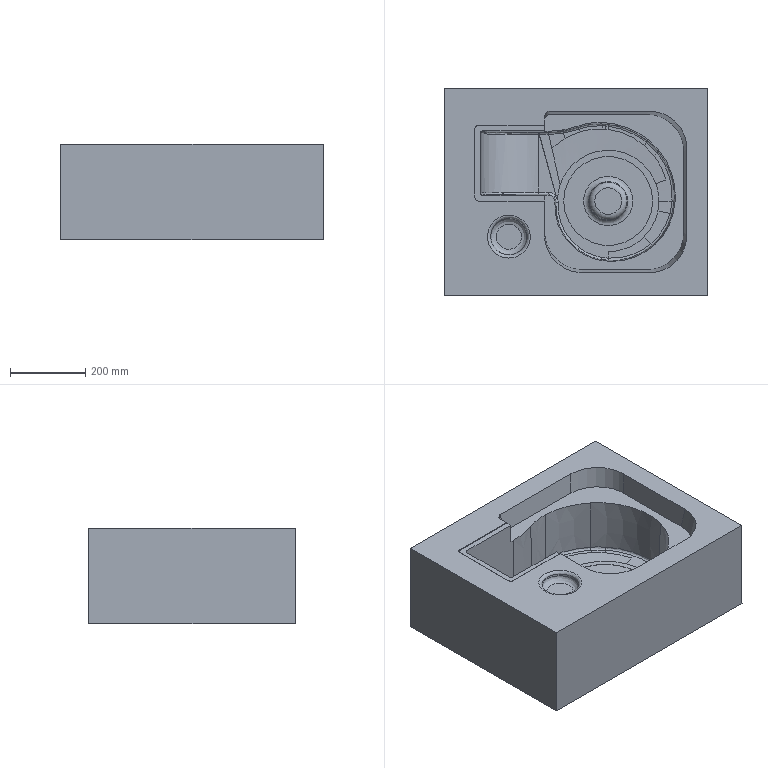NC program | NX | posted with a generic post | part box 700 x 550 x 255 mm
Lines 17668 to 18915 of 43405:
(CAVITY_MILL_COPY_1 , TOOL : D26R0.8)
N35328 M6
N35330 G54
N35332 G17 G0 G90 X-44.068 Y188.604 S1000 M3
N35334 G43 Z30. H0
N35336 Z0.302
N35338 G94 G1 Z-0.698 F1800.
N35340 Y201.604
N35342 X-57.068
N35344 X-68.784
N35346 G3 X-70.358 Y200.391 R1.628
N35348 X-70.433 Y199.808 R2.293
N35350 G1 Y188.61
N35352 Y154.444
N35354 Z0.302
N35356 G0 Z3.
N35358 X-39.123 Y188.506
N35360 Z-0.396
N35362 G1 Z-1.396
N35364 Y201.506
N35366 X-52.123
N35368 X-68.766
N35370 G3 X-70.382 Y200.106 R1.633
N35372 X-70.423 Y199.452 R4.078
N35374 G1 Y184.498
N35376 Y153.351
N35378 Z-0.396
N35380 G0 Z2.302
N35382 X-39.117 Y188.408
N35384 Z-1.094
N35386 G1 Z-2.094
N35388 Y201.408
N35390 X-52.117
N35392 X-68.787
N35394 G3 X-70.356 Y200.026 R1.582
N35396 G1 X-70.408 Y199.618
N35398 X-70.417 Y199.467
N35400 Y184.4
N35402 Y140.492
N35404 Z-1.094
N35406 G0 Z1.604
N35408 X-39.111 Y188.31
N35410 Z-1.792
N35412 G1 Z-2.792
N35414 Y201.31
N35416 X-52.111
N35418 X-68.759
N35420 G3 X-70.37 Y199.838 R1.617
N35422 G1 X-70.411 Y199.386
N35424 Y184.302
N35426 Y139.998
N35428 Z-1.792
N35430 G0 Z0.906
N35432 X-39.105 Y188.212
N35434 Z-2.491
N35436 G1 Z-3.491
N35438 Y201.212
N35440 X-52.105
N35442 X-68.755
N35444 G3 X-70.357 Y199.752 R1.609
N35446 G1 X-70.405 Y199.243
N35448 Y184.204
N35450 Y139.977
N35452 Z-2.491
N35454 G0 Z0.208
N35456 X-39.099 Y188.114
N35458 Z-3.189
N35460 G1 Z-4.189
N35462 Y201.114
N35464 X-52.099
N35466 X-68.745
N35468 G3 X-70.353 Y199.654 R1.615
N35470 G1 X-70.399 Y199.181
N35472 Y184.106
N35474 Y139.965
N35476 Z-3.189
N35478 G0 Z-0.491
N35480 X-39.093 Y188.016
N35482 Z-3.887
N35484 G1 Z-4.887
N35486 Y201.016
N35488 X-52.093
N35490 X-68.749
N35492 G3 X-70.334 Y199.669 R1.606
N35494 X-70.392 Y198.978 R4.518
N35496 G1 Y184.008
N35498 Y139.953
N35500 Z-3.887
N35502 G0 Z-1.189
N35504 X-39.087 Y187.918
N35506 Z-4.585
N35508 G1 Z-5.585
N35510 Y200.918
N35512 X-52.087
N35514 X-68.711
N35516 G3 X-70.358 Y199.38 R1.652
N35518 G1 X-70.386 Y198.974
N35520 Y183.91
N35522 Y139.94
N35524 Z-4.585
N35526 G0 Z-1.887
N35528 X-39.08 Y187.82
N35530 Z-5.283
N35532 G1 Z-6.283
N35534 Y200.82
N35536 X-52.08
N35538 X-68.721
N35540 G3 X-70.33 Y199.468 R1.633
N35542 G1 X-70.349 Y199.357
N35544 X-70.38 Y198.756
N35546 Y183.811
N35548 Y139.928
N35550 Z-5.283
N35552 G0 Z-2.585
N35554 X-39.074 Y187.721
N35556 Z-5.981
N35558 G1 Z-6.981
N35560 Y200.721
N35562 X-52.074
N35564 X-68.709
N35566 G3 X-70.265 Y199.577 R1.63
N35568 G1 X-70.314 Y199.418
N35570 X-70.374 Y198.752
N35572 Y183.713
N35574 Y139.922
N35576 Z-5.981
N35578 G0 Z-3.283
N35580 X-39.068 Y187.623
N35582 Z-6.679
N35584 G1 Z-7.679
N35586 Y200.623
N35588 X-52.068
N35590 X-68.695
N35592 G3 X-70.305 Y199.312 R1.644
N35594 G1 X-70.332 Y199.181
N35596 X-70.368 Y198.583
N35598 Y183.615
N35600 Y139.911
N35602 Z-6.679
N35604 G0 Z-3.981
N35606 X-39.062 Y187.525
N35608 Z-7.377
N35610 G1 Z-8.377
N35612 Y200.525
N35614 X-52.062
N35616 X-68.709
N35618 G3 X-70.316 Y199.062 R1.615
N35620 G1 X-70.362 Y198.579
N35622 Y183.517
N35624 Y139.892
N35626 Z-7.377
N35628 G0 Z-4.679
N35630 X-39.056 Y187.427
N35632 Z-8.076
N35634 G1 Z-9.076
N35636 Y200.427
N35638 X-52.056
N35640 X-68.686
N35642 G3 X-70.289 Y199.1 R1.632
N35644 X-70.356 Y198.378 R3.795
N35646 G1 Y183.419
N35648 Y139.879
N35650 Z-8.076
N35652 G0 Z-5.377
N35654 X-39.05 Y187.329
N35656 Z-8.774
N35658 G1 Z-9.774
N35660 Y200.329
N35662 X-52.05
N35664 X-68.679
N35666 G3 X-70.264 Y199.083 R1.63
N35668 X-70.35 Y198.374 R3.058
N35670 G1 Y183.321
N35672 Y139.867
N35674 Z-8.774
N35676 G0 Z-6.076
N35678 X-39.044 Y187.231
N35680 Z-9.472
N35682 G1 Z-10.472
N35684 Y200.231
N35686 X-52.044
N35688 X-68.677
N35690 G3 X-70.221 Y199.106 R1.622
N35692 X-70.344 Y198.371 R2.564
N35694 G1 Y183.223
N35696 Y139.855
N35698 Z-9.472
N35700 G0 Z-6.774
N35702 X-39.038 Y187.133
N35704 Z-10.17
N35706 G1 Z-11.17
N35708 Y200.133
N35710 X-52.038
N35712 X-68.663
N35714 G3 X-70.268 Y198.777 R1.628
N35716 G1 X-70.338 Y198.367
N35718 Y183.125
N35720 Y139.843
N35722 Z-10.17
N35724 G0 Z-7.472
N35726 X-39.032 Y187.035
N35728 Z-10.868
N35730 G1 Z-11.868
N35732 Y200.035
N35734 X-52.032
N35736 X-68.655
N35738 G3 X-70.256 Y198.746 R1.638
N35740 X-70.332 Y197.924 R3.364
N35742 G1 Y183.027
N35744 Y139.831
N35746 Z-10.868
N35748 G0 Z-8.17
N35750 X-39.026 Y186.937
N35752 Z-11.566
N35754 G1 Z-12.566
N35756 Y199.937
N35758 X-52.026
N35760 X-68.651
N35762 G3 X-70.257 Y198.601 R1.633
N35764 X-70.325 Y197.924 R4.148
N35766 G1 Y182.928
N35768 Y139.818
N35770 Z-11.566
N35772 G0 Z-8.868
N35774 X-39.02 Y186.838
N35776 Z-12.264
N35778 G1 Z-13.264
N35780 Y199.838
N35782 X-52.02
N35784 X-68.643
N35786 G3 X-70.268 Y198.384 R1.635
N35788 G1 X-70.319 Y197.924
N35790 Y182.83
N35792 Y139.806
N35794 Z-12.264
N35796 G0 Z-9.566
N35798 X-39.013 Y186.74
N35800 Z-12.962
N35802 G1 Z-13.962
N35804 Y199.74
N35806 X-52.013
N35808 X-68.637
N35810 G3 X-70.257 Y198.284 R1.63
N35812 G1 X-70.296 Y197.924
N35814 X-70.313 Y197.889
N35816 Y182.732
N35818 Y139.794
N35820 Z-12.962
N35822 G0 Z-10.264
N35824 X-39.007 Y186.642
N35826 Z-13.66
N35828 G1 Z-14.66
N35830 Y199.642
N35832 X-52.007
N35834 X-68.631
N35836 G3 X-70.243 Y198.242 R1.628
N35838 G1 X-70.307 Y197.789
N35840 Y182.634
N35842 Y139.782
N35844 Z-13.66
N35846 G0 Z-10.962
N35848 X-39.001 Y186.544
N35850 Z-14.359
N35852 G1 Z-15.359
N35854 Y199.544
N35856 X-52.001
N35858 X-68.614
N35860 G3 X-70.236 Y198.139 R1.639
N35862 G1 X-70.301 Y197.69
N35864 Y182.536
N35866 Y139.77
N35868 Z-14.359
N35870 G0 Z-11.66
N35872 X-38.995 Y186.446
N35874 Z-15.057
N35876 G1 Z-16.057
N35878 Y199.446
N35880 X-51.995
N35882 X-68.653
N35884 G3 X-70.198 Y198.147 R1.568
N35886 G1 X-70.295 Y197.59
N35888 Y182.438
N35890 Y139.758
N35892 Z-15.057
N35894 G0 Z-12.359
N35896 X-38.989 Y186.348
N35898 Z-15.755
N35900 G1 Z-16.755
N35902 Y199.348
N35904 X-51.989
N35906 X-68.507
N35908 G3 X-70.054 Y198.463 R1.634
N35910 X-70.289 Y197.491 R2.485
N35912 G1 Y182.34
N35914 Y139.745
N35916 Z-15.755
N35918 G0 Z-13.057
N35920 X-38.983 Y186.25
N35922 Z-16.453
N35924 G1 Z-17.453
N35926 Y199.25
N35928 X-51.983
N35930 X-68.606
N35932 G3 X-70.077 Y198.296 R1.611
N35934 G1 X-70.086 Y198.276
N35936 G3 X-70.283 Y197.391 R1.86
N35938 G1 Y182.242
N35940 Y139.733
N35942 Z-16.453
N35944 G0 Z-13.755
N35946 X-38.977 Y186.152
N35948 Z-17.151
N35950 G1 Z-18.151
N35952 Y199.152
N35954 X-51.977
N35956 X-68.494
N35958 G3 X-70.044 Y198.26 R1.634
N35960 X-70.277 Y197.292 R1.961
N35962 G1 Y182.144
N35964 Y139.721
N35966 Z-17.151
N35968 G0 Z-14.453
N35970 X-38.971 Y186.054
N35972 Z-17.849
N35974 G1 Z-18.849
N35976 Y199.054
N35978 X-51.971
N35980 X-68.488
N35982 G3 X-70.132 Y197.924 R1.623
N35984 X-70.271 Y197.192 R1.509
N35986 G1 Y182.045
N35988 Y139.709
N35990 Z-17.849
N35992 G0 Z-15.151
N35994 X-38.965 Y185.955
N35996 Z-18.547
N35998 G1 Z-19.547
N36000 Y198.955
N36002 X-51.965
N36004 X-68.482
N36006 G3 X-69.579 Y198.623 R1.753
N36008 X-70.264 Y197.093 R1.952
N36010 G1 Y181.947
N36012 Y139.697
N36014 Z-18.547
N36016 G0 Z-15.849
N36018 X-38.959 Y185.857
N36020 Z-19.245
N36022 G1 Z-20.245
N36024 Y198.857
N36026 X-51.959
N36028 X-68.598
N36030 G3 X-69.901 Y198.173 R1.583
N36032 X-70.258 Y196.994 R2.026
N36034 G1 Y181.849
N36036 Y139.691
N36038 Z-19.245
N36040 G0 Z-16.547
N36042 X-38.953 Y185.759
N36044 Z-19.943
N36046 G1 Z-20.943
N36048 Y198.759
N36050 X-51.953
N36052 X-68.545
N36054 G3 X-70.206 Y197.285 R1.673
N36056 G1 X-70.252 Y196.894
N36058 Y181.751
N36060 Y139.68
N36062 Z-19.943
N36064 G0 Z-17.245
N36066 X-38.946 Y185.661
N36068 Z-20.642
N36070 G1 Z-21.642
N36072 Y198.661
N36074 X-51.946
N36076 X-68.554
N36078 G3 X-70.198 Y197.162 R1.65
N36080 G1 X-70.231 Y196.795
N36082 X-70.246 Y196.667
N36084 Y181.653
N36086 Y139.66
N36088 Z-20.642
N36090 G0 Z-17.943
N36092 X-38.94 Y185.563
N36094 Z-21.34
N36096 G1 Z-22.34
N36098 Y198.563
N36100 X-51.94
N36102 X-68.547
N36104 G3 X-70.191 Y197.063 R1.651
N36106 G1 X-70.225 Y196.695
N36108 X-70.24 Y196.667
N36110 Y181.555
N36112 Y139.648
N36114 Z-21.34
N36116 G0 Z-18.642
N36118 X-38.934 Y185.465
N36120 Z-22.038
N36122 G1 Z-23.038
N36124 Y198.465
N36126 X-51.934
N36128 X-68.534
N36130 G3 X-70.186 Y196.967 R1.66
N36132 G1 X-70.215 Y196.667
N36134 X-70.234 Y196.575
N36136 Y181.457
N36138 Y139.636
N36140 Z-22.038
N36142 G0 Z-19.34
N36144 X-38.928 Y185.367
N36146 Z-22.736
N36148 G1 Z-23.736
N36150 Y198.367
N36152 X-51.928
N36154 X-68.555
N36156 G3 X-70.176 Y196.925 R1.632
N36158 G1 X-70.228 Y196.48
N36160 Y181.359
N36162 Y139.624
N36164 Z-22.736
N36166 G0 Z-20.038
N36168 X-38.922 Y185.269
N36170 Z-23.434
N36172 G1 Z-24.434
N36174 Y198.269
N36176 X-51.922
N36178 X-68.547
N36180 G3 X-70.169 Y196.828 R1.633
N36182 G1 X-70.222 Y196.384
N36184 Y181.261
N36186 Y139.611
N36188 Z-23.434
N36190 G0 Z-20.736
N36192 X-38.916 Y185.171
N36194 Z-24.132
N36196 G1 Z-25.132
N36198 Y198.171
N36200 X-51.916
N36202 X-68.433
N36204 G3 X-70.174 Y196.667 R1.668
N36206 G1 X-70.216 Y196.289
N36208 Y181.162
N36210 Y139.599
N36212 Z-24.132
N36214 G0 Z-21.434
N36216 X-38.91 Y185.072
N36218 Z-24.83
N36220 G1 Z-25.83
N36222 Y198.072
N36224 X-51.91
N36226 X-68.427
N36228 G3 X-70.161 Y196.639 R1.67
N36230 G1 X-70.21 Y196.193
N36232 Y181.064
N36234 Y139.587
N36236 Z-24.83
N36238 G0 Z-22.132
N36240 X-38.904 Y184.974
N36242 Z-25.528
N36244 G1 Z-26.528
N36246 Y197.974
N36248 X-51.904
N36250 X-68.522
N36252 G3 X-70.061 Y196.884 R1.631
N36254 X-70.204 Y196.098 R2.538
N36256 G1 Y180.966
N36258 Y139.575
N36260 Z-25.528
N36262 G0 Z-22.83
N36264 X-38.898 Y184.876
N36266 Z-26.227
N36268 G1 Z-27.227
N36270 Y197.876
N36272 X-51.898
N36274 X-68.51
N36276 G3 X-70.064 Y196.753 R1.637
N36278 X-70.197 Y196.003 R2.655
N36280 G1 Y180.868
N36282 Y139.563
N36284 Z-26.227
N36286 G0 Z-23.528
N36288 X-38.892 Y184.778
N36290 Z-26.925
N36292 G1 Z-27.925
N36294 Y197.778
N36296 X-51.892
N36298 X-68.508
N36300 G3 X-70.055 Y196.665 R1.632
N36302 X-70.191 Y195.907 R2.639
N36304 G1 Y180.77
N36306 Y139.55
N36308 Z-26.925
N36310 G0 Z-24.227
N36312 X-38.886 Y184.68
N36314 Z-27.623
N36316 G1 Z-28.623
N36318 Y197.68
N36320 X-51.886
N36322 X-68.5
N36324 G3 X-70.048 Y196.575 R1.637
N36326 X-70.185 Y195.812 R2.55
N36328 G1 Y180.672
N36330 Y139.538
N36332 Z-27.623
N36334 G0 Z-24.925
N36336 X-38.879 Y184.582
N36338 Z-28.321
N36340 G1 Z-29.321
N36342 Y197.582
N36344 X-51.879
N36346 X-68.397
N36348 G3 X-69.998 Y196.596 R1.654
N36350 X-70.179 Y195.716 R2.546
N36352 G1 Y180.574
N36354 Y139.526
N36356 Z-28.321
N36358 G0 Z-25.623
N36360 X-38.873 Y184.484
N36362 Z-29.019
N36364 G1 Z-30.019
N36366 Y197.484
N36368 X-51.873
N36370 X-68.482
N36372 G3 X-70.046 Y196.35 R1.647
N36374 X-70.173 Y195.621 R2.564
N36376 G1 Y180.476
N36378 Y139.514
N36380 Z-29.019
N36382 G0 Z-26.321
N36384 X-38.867 Y184.386
N36386 Z-29.717
N36388 G1 Z-30.717
N36390 Y197.386
N36392 X-51.867
N36394 X-68.475
N36396 G3 X-70.045 Y196.24 R1.649
N36398 X-70.167 Y195.411 R2.568
N36400 G1 Y180.377
N36402 Y139.502
N36404 Z-29.717
N36406 G0 Z-27.019
N36408 X-38.861 Y184.287
N36410 Z-30.415
N36412 G1 Z-31.415
N36414 Y197.287
N36416 X-51.861
N36418 X-68.379
N36420 G3 X-69.998 Y196.263 R1.661
N36422 X-70.161 Y195.411 R2.598
N36424 G1 Y180.279
N36426 Y139.489
N36428 Z-30.415
N36430 G0 Z-27.717
N36432 X-38.855 Y184.189
N36434 Z-31.113
N36436 G1 Z-32.113
N36438 Y197.189
N36440 X-51.855
N36442 X-68.372
N36444 G3 X-70.106 Y195.762 R1.676
N36446 G1 X-70.155 Y195.244
N36448 Y180.181
N36450 Y139.477
N36452 Z-31.113
N36454 G0 Z-28.415
N36456 X-38.849 Y184.091
N36458 Z-31.811
N36460 G1 Z-32.811
N36462 Y197.091
N36464 X-51.849
N36466 X-68.366
N36468 G3 X-70.1 Y195.664 R1.674
N36470 G1 X-70.149 Y195.158
N36472 Y180.083
N36474 Y139.465
N36476 Z-31.811
N36478 G0 Z-29.113
N36480 X-38.843 Y183.993
N36482 Z-32.51
N36484 G1 Z-33.51
N36486 Y196.993
N36488 X-51.843
N36490 X-68.36
N36492 G3 X-70.094 Y195.567 R1.674
N36494 G1 X-70.132 Y195.156
N36496 X-70.143 Y195.072
N36498 Y179.985
N36500 Y139.453
N36502 Z-32.51
N36504 G0 Z-29.811
N36506 X-38.837 Y183.895
N36508 Z-33.208
N36510 G1 Z-34.208
N36512 Y196.895
N36514 X-51.837
N36516 X-68.354
N36518 G3 X-70.088 Y195.469 R1.671
N36520 G1 X-70.137 Y195.002
N36522 Y179.887
N36524 Y139.441
N36526 Z-33.208
N36528 G0 Z-30.51
N36530 X-38.831 Y183.797
N36532 Z-33.906
N36534 G1 Z-34.906
N36536 Y196.797
N36538 X-51.831
N36540 X-68.348
N36542 G3 X-70.072 Y195.411 R1.663
N36544 G1 X-70.13 Y195.
N36546 Y179.789
N36548 Y139.429
N36550 Z-33.906
N36552 G0 Z-31.208
N36554 X-38.825 Y183.699
N36556 Z-34.604
N36558 G1 Z-35.604
N36560 Y196.699
N36562 X-51.825
N36564 X-68.46
N36566 G3 X-70.057 Y195.3 R1.61
N36568 G1 X-70.124 Y194.791
N36570 Y179.691
N36572 Y139.416
N36574 Z-34.604
N36576 G0 Z-31.906
N36578 X-38.819 Y183.601
N36580 Z-35.302
N36582 G1 Z-36.302
N36584 Y196.601
N36586 X-51.819
N36588 X-68.43
N36590 G3 X-70.042 Y195.208 R1.628
N36592 G1 X-70.118 Y194.685
N36594 Y179.593
N36596 Y139.404
N36598 Z-35.302
N36600 G0 Z-32.604
N36602 X-38.812 Y183.503
N36604 Z-36.
N36606 G1 Z-37.
N36608 Y196.503
N36610 X-51.812
N36612 X-68.33
N36614 G3 X-70.063 Y194.993 R1.646
N36616 G1 X-70.112 Y194.631
N36618 Y179.494
N36620 Y139.392
N36622 Z-36.
N36624 G0 Z-33.302
N36626 X-38.806 Y183.404
N36628 Z-36.698
N36630 G1 Z-37.698
N36632 Y196.404
N36634 X-51.806
N36636 X-68.324
N36638 G3 X-70.043 Y194.99 R1.64
N36640 G1 X-70.106 Y194.502
N36642 Y179.396
N36644 Y139.38
N36646 Z-36.698
N36648 G0 Z-34.
N36650 X-38.8 Y183.306
N36652 Z-37.396
N36654 G1 Z-38.396
N36656 Y196.306
N36658 X-51.8
N36660 X-68.417
N36662 G3 X-70.035 Y194.897 R1.633
N36664 G1 X-70.1 Y194.424
N36666 Y179.298
N36668 Y139.368
N36670 Z-37.396
N36672 G0 Z-34.698
N36674 X-38.794 Y183.208
N36676 Z-38.095
N36678 G1 Z-39.095
N36680 Y196.208
N36682 X-51.794
N36684 X-68.403
N36686 G3 X-70.027 Y194.804 R1.641
N36688 G1 X-70.094 Y194.346
N36690 Y179.2
N36692 Y139.355
N36694 Z-38.095
N36696 G0 Z-35.396
N36698 X-38.788 Y183.11
N36700 Z-38.793
N36702 G1 Z-39.793
N36704 Y196.11
N36706 X-51.788
N36708 X-68.404
N36710 G3 X-70.028 Y194.679 R1.637
N36712 G1 X-70.088 Y194.211
N36714 Y179.102
N36716 Y139.343
N36718 Z-38.793
N36720 G0 Z-36.095
N36722 X-38.782 Y183.012
N36724 Z-39.491
N36726 G1 Z-40.491
N36728 Y196.012
N36730 X-51.782
N36732 X-68.299
N36734 G3 X-70.037 Y194.492 R1.652
N36736 G1 X-70.082 Y194.121
N36738 Y179.004
N36740 Y139.331
N36742 Z-39.491
N36744 G0 Z-36.793
N36746 X-38.776 Y182.914
N36748 Z-40.189
N36750 G1 Z-41.189
N36752 Y195.914
N36754 X-51.776
N36756 X-68.394
N36758 G3 X-70.02 Y194.496 R1.641
N36760 G1 X-70.021 Y194.49
N36762 X-70.038 Y194.415
N36764 X-70.076 Y194.02
N36766 Y178.906
N36768 Y139.319
N36770 Z-40.189
N36772 G0 Z-37.491
N36774 X-38.77 Y182.816
N36776 Z-40.887
N36778 G1 Z-41.887
N36780 Y195.816
N36782 X-51.77
N36784 X-68.287
N36786 G3 X-70.033 Y194.261 R1.658
N36788 G1 X-70.07 Y193.952
N36790 Y178.808
N36792 Y139.307
N36794 Z-40.887
N36796 G0 Z-38.189
N36798 X-38.764 Y182.718
N36800 Z-41.585
N36802 G1 Z-42.585
N36804 Y195.718
N36806 X-51.764
N36808 X-68.281
N36810 G3 X-70.017 Y194.259 R1.649
N36812 G1 X-70.063 Y193.824
N36814 Y178.71
N36816 Y139.295
N36818 Z-41.585
N36820 G0 Z-38.887
N36822 X-38.758 Y182.62
N36824 Z-42.283
N36826 G1 Z-43.283
N36828 Y195.62
N36830 X-51.758
N36832 X-68.275
N36834 G3 X-70.014 Y194.154 R1.654
N36836 G1 X-70.057 Y193.762
N36838 Y178.611
N36840 Y139.282
N36842 Z-42.283
N36844 G0 Z-39.585
N36846 X-38.752 Y182.521
N36848 Z-42.981
N36850 G1 Z-43.981
N36852 Y195.521
N36854 X-51.752
N36856 X-68.386
N36858 G3 X-69.828 Y194.615 R1.601
N36860 X-70.051 Y193.639 R2.254
N36862 G1 Y178.513
N36864 Y139.27
N36866 Z-42.981
N36868 G0 Z-40.283
N36870 X-38.745 Y182.423
N36872 Z-43.679
N36874 G1 Z-44.679
N36876 Y195.423
N36878 X-51.745
N36880 X-68.263
N36882 G3 X-70.015 Y193.883 R1.664
N36884 G1 X-70.045 Y193.512
N36886 Y178.415
N36888 Y139.258
N36890 Z-43.679
N36892 G0 Z-40.981
N36894 X-38.739 Y182.325
N36896 Z-44.378
N36898 G1 Z-45.378
N36900 Y195.325
N36902 X-51.739
N36904 X-68.366
N36906 G3 X-69.931 Y194.158 R1.633
N36908 X-70.039 Y193.449 R2.598
N36910 G1 Y178.317
N36912 Y139.246
N36914 Z-44.378
N36916 G0 Z-41.679
N36918 X-38.733 Y182.227
N36920 Z-45.076
N36922 G1 Z-46.076
N36924 Y195.227
N36926 X-51.733
N36928 X-68.25
N36930 G3 X-69.998 Y193.789 R1.666
N36932 G1 X-70.033 Y193.387
N36934 Y178.219
N36936 Y139.234
N36938 Z-45.076
N36940 G0 Z-42.378
N36942 X-38.727 Y182.129
N36944 Z-45.774
N36946 G1 Z-46.774
N36948 Y195.129
N36950 X-51.727
N36952 X-68.345
N36954 G3 X-69.973 Y193.773 R1.656
N36956 G1 X-69.998 Y193.639
N36958 X-70.027 Y193.229
N36960 Y178.121
N36962 Y139.221
N36964 Z-45.774
N36966 G0 Z-43.076
N36968 X-38.721 Y182.031
N36970 Z-46.472
N36972 G1 Z-47.472
N36974 Y195.031
N36976 X-51.721
N36978 X-68.347
N36980 G3 X-69.968 Y193.615 R1.637
N36982 G1 X-70.021 Y193.229
N36984 Y178.023
N36986 Y139.209
N36988 Z-46.472
N36990 G0 Z-43.774
N36992 X-38.715 Y181.933
N36994 Z-47.17
N36996 G1 Z-48.17
N36998 Y194.933
N37000 X-51.715
N37002 X-68.342
N37004 G3 X-69.931 Y193.69 R1.637
N37006 X-70.015 Y193.025 R2.846
N37008 G1 Y177.925
N37010 Y139.197
N37012 Z-47.17
N37014 G0 Z-44.472
N37016 X-38.709 Y181.835
N37018 Z-47.868
N37020 G1 Z-48.868
N37022 Y194.835
N37024 X-51.709
N37026 X-68.332
N37028 G3 X-69.965 Y193.386 R1.644
N37030 G1 X-70.009 Y193.024
N37032 Y177.827
N37034 Y139.185
N37036 Z-47.868
N37038 G0 Z-45.17
N37040 X-38.703 Y181.737
N37042 Z-48.566
N37044 G1 Z-49.566
N37046 Y194.737
N37048 X-51.703
N37050 X-68.369
N37052 G3 X-69.906 Y193.46 R1.564
N37054 G1 X-69.998 Y192.973
N37056 X-70.003 Y192.897
N37058 Y177.728
N37060 Y139.173
N37062 Z-48.566
N37064 G0 Z3.
N37066 X-57.9 Y172.249
N37068 Z0.302
N37070 G1 Z-0.698
N37072 X-79.312 Y164.576
N37074 G2 X-83.957 Y163.792 R13.398
N37076 G1 X-256.512
N37078 Y-10.819
N37080 X-83.845
N37082 G2 X-79.452 Y-11.561 R13.419
N37084 G1 X-57.953 Y-19.024
N37086 Z0.302
N37088 G0 Z3.
N37090 X-57.281 Y184.446
N37092 Z-0.396
N37094 G1 Z-1.396
N37096 X-68.289 Y187.538
N37098 X-70.645 Y174.753
N37100 G2 X-83.823 Y163.781 R13.4
N37102 G1 X-256.502
N37104 Y-10.808
N37106 X-83.823
N37108 G2 X-70.641 Y-21.802 R13.4
N37110 G1 X-68.307 Y-34.591
N37112 X-57.423
N37114 Z-0.396
N37116 G0 Z30.
N37118 X-215.552 Y136.769
N37120 Z-1.094
N37122 G1 Z-2.094
N37124 Y149.769
N37126 X-228.552
N37128 X-241.536
N37130 Y136.786
N37132 Y123.786
N37134 X-228.536
N37136 Z-1.094
N37138 G0 Z1.604
N37140 X-211.773 Y136.342
N37142 Z-1.792
N37144 G1 Z-2.792
N37146 Y149.342
N37148 X-224.773
N37150 X-241.108
N37152 Y133.007
N37154 Y120.007
N37156 X-228.108
N37158 Z-1.792
N37160 G0 Z0.906
N37162 X-211.127 Y136.323
N37164 Z-2.491
N37166 G1 Z-3.491
N37168 Y149.323
N37170 X-224.127
N37172 X-241.09
N37174 Y132.36
N37176 Y119.36
N37178 X-228.09
N37180 Z-2.491
N37182 G0 Z0.208
N37184 X-211.115 Y136.311
N37186 Z-3.189
N37188 G1 Z-4.189
N37190 Y149.311
N37192 X-224.115
N37194 X-241.078
N37196 Y132.348
N37198 Y119.348
N37200 X-228.078
N37202 Z-3.189
N37204 G0 Z-0.491
N37206 X-211.103 Y136.299
N37208 Z-3.887
N37210 G1 Z-4.887
N37212 Y149.299
N37214 X-224.103
N37216 X-241.066
N37218 Y132.336
N37220 Y119.336
N37222 X-228.066
N37224 Z-3.887
N37226 G0 Z-1.189
N37228 X-211.09 Y136.287
N37230 Z-4.585
N37232 G1 Z-5.585
N37234 Y149.287
N37236 X-224.09
N37238 X-241.053
N37240 Y132.324
N37242 Y119.324
N37244 X-228.053
N37246 Z-4.585
N37248 G0 Z-1.887
N37250 X-211.078 Y136.275
N37252 Z-5.283
N37254 G1 Z-6.283
N37256 Y149.275
N37258 X-224.078
N37260 X-241.041
N37262 Y132.312
N37264 Y119.312
N37266 X-228.041
N37268 Z-5.283
N37270 G0 Z-2.585
N37272 X-211.066 Y136.262
N37274 Z-5.981
N37276 G1 Z-6.981
N37278 Y149.262
N37280 X-224.066
N37282 X-241.029
N37284 Y132.299
N37286 Y119.299
N37288 X-228.029
N37290 Z-5.981
N37292 G0 Z-3.283
N37294 X-211.054 Y136.25
N37296 Z-6.679
N37298 G1 Z-7.679
N37300 Y149.25
N37302 X-224.054
N37304 X-241.017
N37306 Y132.287
N37308 Y119.287
N37310 X-228.017
N37312 Z-6.679
N37314 G0 Z-3.981
N37316 X-211.042 Y136.238
N37318 Z-7.377
N37320 G1 Z-8.377
N37322 Y149.238
N37324 X-224.042
N37326 X-241.005
N37328 Y132.275
N37330 Y119.275
N37332 X-228.005
N37334 Z-7.377
N37336 G0 Z-4.679
N37338 X-211.03 Y136.226
N37340 Z-8.076
N37342 G1 Z-9.076
N37344 Y149.226
N37346 X-224.03
N37348 X-240.993
N37350 Y132.263
N37352 Y119.263
N37354 X-227.993
N37356 Z-8.076
N37358 G0 Z-5.377
N37360 X-211.017 Y136.214
N37362 Z-8.774
N37364 G1 Z-9.774
N37366 Y149.214
N37368 X-224.017
N37370 X-240.98
N37372 Y132.251
N37374 Y119.251
N37376 X-227.98
N37378 Z-8.774
N37380 G0 Z-6.076
N37382 X-211.005 Y136.202
N37384 Z-9.472
N37386 G1 Z-10.472
N37388 Y149.202
N37390 X-224.005
N37392 X-240.968
N37394 Y132.239
N37396 Y119.239
N37398 X-227.968
N37400 Z-9.472
N37402 G0 Z-6.774
N37404 X-210.993 Y136.189
N37406 Z-10.17
N37408 G1 Z-11.17
N37410 Y149.189
N37412 X-223.993
N37414 X-240.956
N37416 Y132.226
N37418 Y119.226
N37420 X-227.956
N37422 Z-10.17
N37424 G0 Z-7.472
N37426 X-210.981 Y136.177
N37428 Z-10.868
N37430 G1 Z-11.868
N37432 Y149.177
N37434 X-223.981
N37436 X-240.944
N37438 Y132.214
N37440 Y119.214
N37442 X-227.944
N37444 Z-10.868
N37446 G0 Z-8.17
N37448 X-210.969 Y136.165
N37450 Z-11.566
N37452 G1 Z-12.566
N37454 Y149.165
N37456 X-223.969
N37458 X-240.932
N37460 Y132.202
N37462 Y119.202
N37464 X-227.932
N37466 Z-11.566
N37468 G0 Z-8.868
N37470 X-210.956 Y136.153
N37472 Z-12.264
N37474 G1 Z-13.264
N37476 Y149.153
N37478 X-223.956
N37480 X-240.919
N37482 Y132.19
N37484 Y119.19
N37486 X-227.919
N37488 Z-12.264
N37490 G0 Z-9.566
N37492 X-210.944 Y136.141
N37494 Z-12.962
N37496 G1 Z-13.962
N37498 Y149.141
N37500 X-223.944
N37502 X-240.907
N37504 Y132.178
N37506 Y119.178
N37508 X-227.907
N37510 Z-12.962
N37512 G0 Z-10.264
N37514 X-210.932 Y136.128
N37516 Z-13.66
N37518 G1 Z-14.66
N37520 Y149.128
N37522 X-223.932
N37524 X-240.895
N37526 Y132.165
N37528 Y119.165
N37530 X-227.895
N37532 Z-13.66
N37534 G0 Z-10.962
N37536 X-210.92 Y136.116
N37538 Z-14.359
N37540 G1 Z-15.359
N37542 Y149.116
N37544 X-223.92
N37546 X-240.883
N37548 Y132.153
N37550 Y119.153
N37552 X-227.883
N37554 Z-14.359
N37556 G0 Z-11.66
N37558 X-210.908 Y136.104
N37560 Z-15.057
N37562 G1 Z-16.057
N37564 Y149.104
N37566 X-223.908
N37568 X-240.871
N37570 Y132.141
N37572 Y119.141
N37574 X-227.871
N37576 Z-15.057
N37578 G0 Z-12.359
N37580 X-210.895 Y136.092
N37582 Z-15.755
N37584 G1 Z-16.755
N37586 Y149.092
N37588 X-223.895
N37590 X-240.858
N37592 Y132.129
N37594 Y119.129
N37596 X-227.858
N37598 Z-15.755
N37600 G0 Z-13.057
N37602 X-210.883 Y136.08
N37604 Z-16.453
N37606 G1 Z-17.453
N37608 Y149.08
N37610 X-223.883
N37612 X-240.846
N37614 Y132.117
N37616 Y119.117
N37618 X-227.846
N37620 Z-16.453
N37622 G0 Z-13.755
N37624 X-210.871 Y136.067
N37626 Z-17.151
N37628 G1 Z-18.151
N37630 Y149.067
N37632 X-223.871
N37634 X-240.834
N37636 Y132.104
N37638 Y119.104
N37640 X-227.834
N37642 Z-17.151
N37644 G0 Z-14.453
N37646 X-210.859 Y136.055
N37648 Z-17.849
N37650 G1 Z-18.849
N37652 Y149.055
N37654 X-223.859
N37656 X-240.822
N37658 Y132.092
N37660 Y119.092
N37662 X-227.822
N37664 Z-17.849
N37666 G0 Z-15.151
N37668 X-210.847 Y136.043
N37670 Z-18.547
N37672 G1 Z-19.547
N37674 Y149.043
N37676 X-223.847
N37678 X-240.81
N37680 Y132.08
N37682 Y119.08
N37684 X-227.81
N37686 Z-18.547
N37688 G0 Z-15.849
N37690 X-210.835 Y136.031
N37692 Z-19.245
N37694 G1 Z-20.245
N37696 Y149.031
N37698 X-223.835
N37700 X-240.798
N37702 Y132.068
N37704 Y119.068
N37706 X-227.798
N37708 Z-19.245
N37710 G0 Z-16.547
N37712 X-210.822 Y136.019
N37714 Z-19.943
N37716 G1 Z-20.943
N37718 Y149.019
N37720 X-223.822
N37722 X-240.785
N37724 Y132.056
N37726 Y119.056
N37728 X-227.785
N37730 Z-19.943
N37732 G0 Z-17.245
N37734 X-210.81 Y136.007
N37736 Z-20.642
N37738 G1 Z-21.642
N37740 Y149.007
N37742 X-223.81
N37744 X-240.773
N37746 Y132.044
N37748 Y119.044
N37750 X-227.773
N37752 Z-20.642
N37754 G0 Z-17.943
N37756 X-210.798 Y135.994
N37758 Z-21.34
N37760 G1 Z-22.34
N37762 Y148.994
N37764 X-223.798
N37766 X-240.761
N37768 Y132.031
N37770 Y119.031
N37772 X-227.761
N37774 Z-21.34
N37776 G0 Z-18.642
N37778 X-210.786 Y135.982
N37780 Z-22.038
N37782 G1 Z-23.038
N37784 Y148.982
N37786 X-223.786
N37788 X-240.749
N37790 Y132.019
N37792 Y119.019
N37794 X-227.749
N37796 Z-22.038
N37798 G0 Z-19.34
N37800 X-210.774 Y135.97
N37802 Z-22.736
N37804 G1 Z-23.736
N37806 Y148.97
N37808 X-223.774
N37810 X-240.737
N37812 Y132.007
N37814 Y119.007
N37816 X-227.737